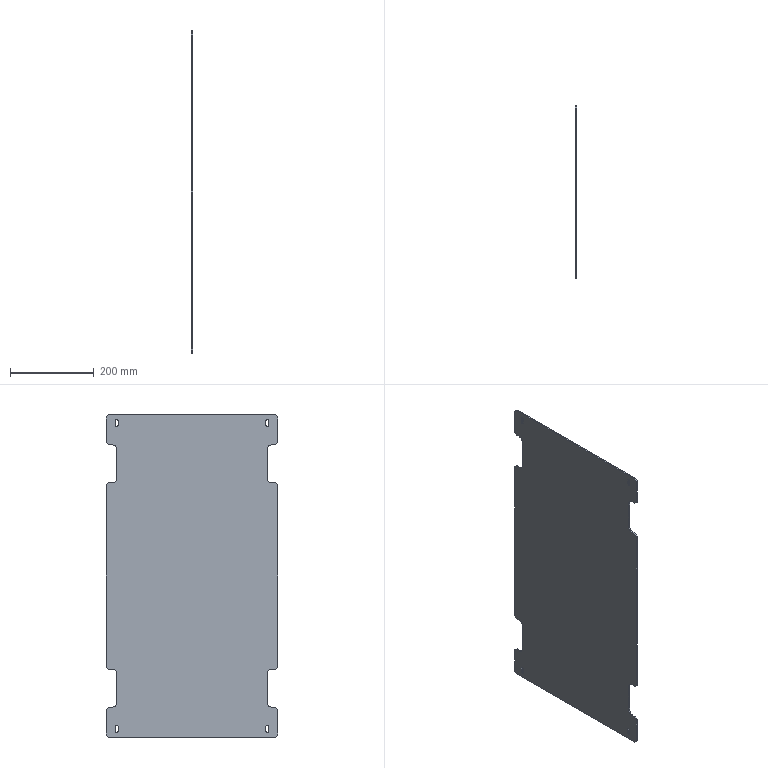Part | SolidWorks | features BaseBody 1 | 1 solid | 62 faces | box 3 x 410 x 770 mm | volume 918863 mm3 | plane 42 | cylinder 20 | commonest cylinder face diameters 7 x12 20 x8